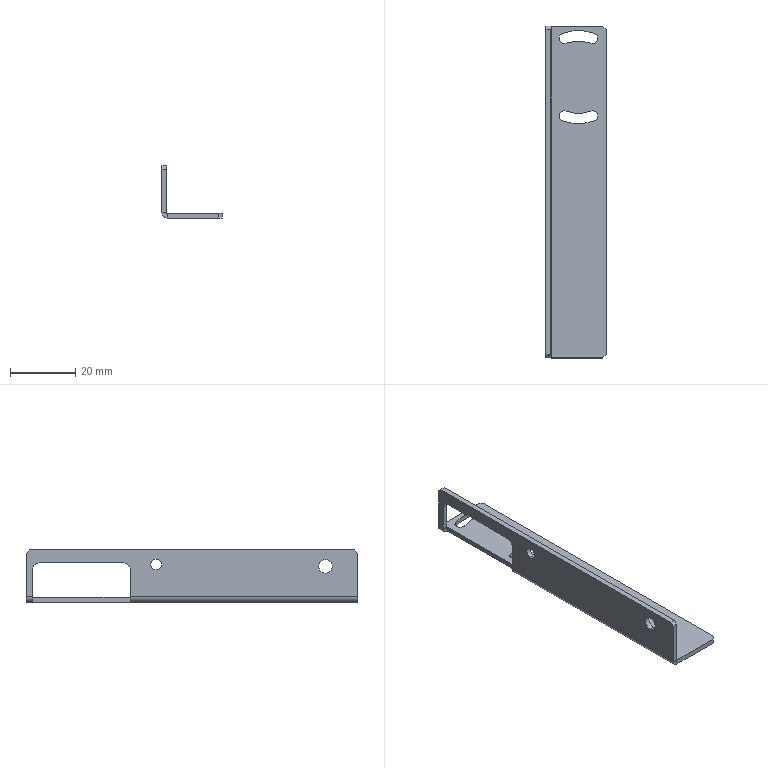Part | STEP file | CX440 adjusting plate 2_powder-coated matt silver grey | 1 solid | 44 faces | box 18.5 x 102 x 16 mm | volume 4317 mm3 | plane 24 | cylinder 20 | commonest cylinder face diameters 3.2 x8 0.2 x2 3.3 x2 4 x2 4.2 x2 22.2 x2